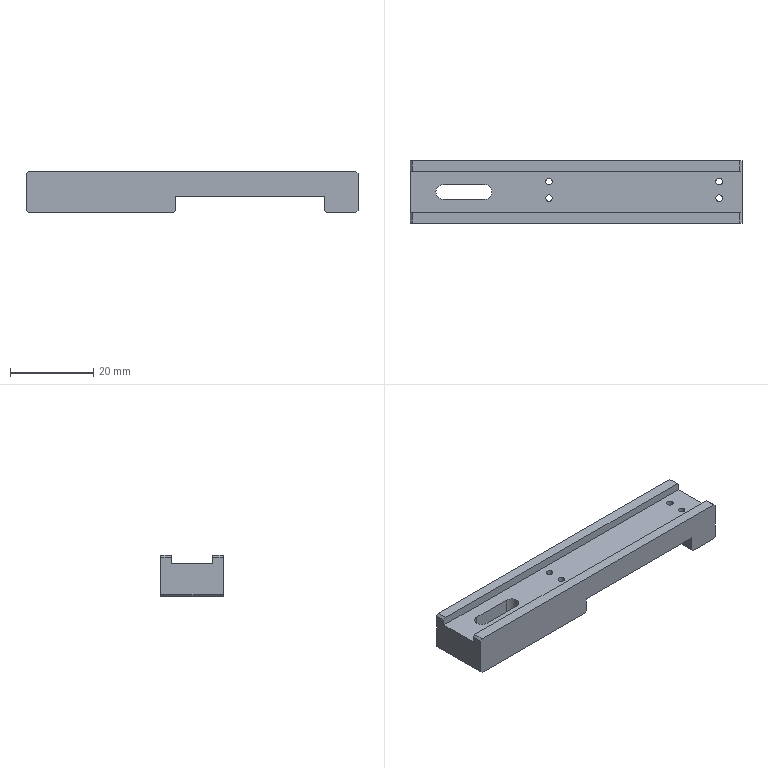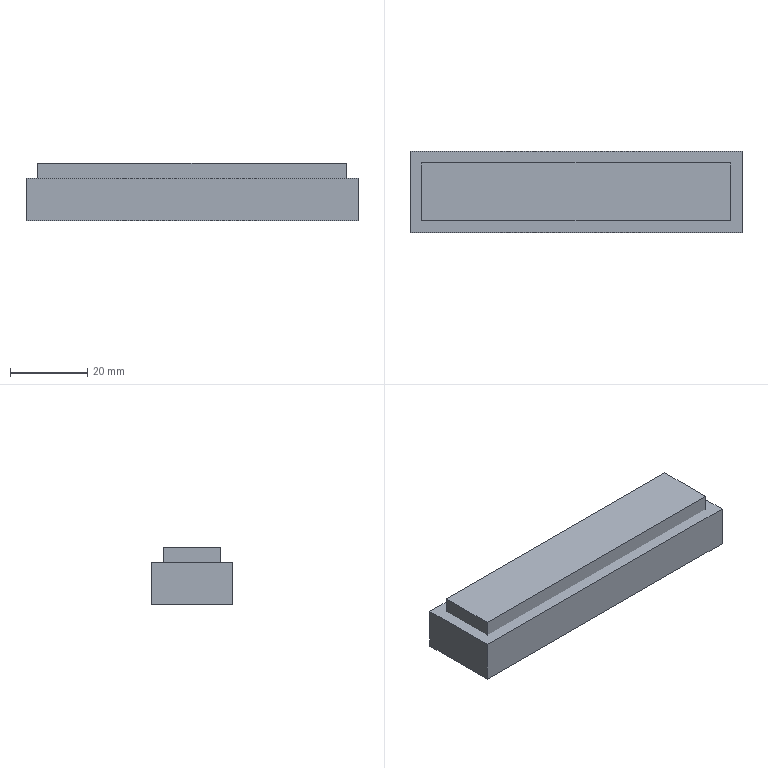CAM job | NX | 3-axis milling, drilling | part box 80 x 15 x 10 mm | stock box 86 x 21 x 15 mm
Tools:
number,name,description,diameter,corner_radius,flute_length,length,flutes
3,D63,Milling Tool-5 Parameters,63.0,0.0,50.0,75.0,2
4,D10,Milling Tool-5 Parameters,10.0,0.0,50.0,75.0,2
14,D10JING,Milling Tool-5 Parameters,10.0,0.0,50.0,75.0,2
1,D6A45,Milling Tool-5 Parameters,6.0,0.0,50.0,75.0,2
24,1.6ZT,Drilling Tool,1.6,0.0,35.0,50.0,2
17,D3,Milling Tool-5 Parameters,3.0,0.0,50.0,75.0,2
16,D6,Milling Tool-5 Parameters,6.0,0.0,50.0,75.0,2
Operations:
program,operation,operation_type,tool,method,geometry_group,spindle_rpm,surface_speed,feed_per_tooth,feed_cut,feed_plunge,cut_length_mm,path_length_mm,cut_time_min,machine_time_min
1,FLOOR_WALL,VolumeBased25DMillingOperation,D63,METHOD,A,6500.0,1286.0,0.1154,1500.0,100.0,161.0,215.0,0.1073,0.1127
1,DRILLING,Operation,D6A45,METHOD,A,5000.0,94.0,0.025,250.0,0.0,16.2,152.51,0.0648,0.0784
1,DRILLING_COPY_1_COPY,Operation,1.6ZT,METHOD,A,2000.0,37.0,0.0375,150.0,0.0,51.923,223.955,0.3462,0.3634
1,ADAPTIVE_MILLING,CavityMilling,D10,METHOD,A,7500.0,235.0,0.2,3000.0,1000.0,2724.517,2881.399,0.9122,0.9279
1,ZLEVEL_PROFILE,ZLevelMilling,D10JING,METHOD,A,7500.0,235.0,0.0667,1000.0,100.0,228.754,306.754,0.2288,0.2366
1,FLOOR_WALL_1_COPY_COPY,VolumeBased25DMillingOperation,D10JING,METHOD,A,7500.0,235.0,0.08,1200.0,1000.0,260.997,473.497,0.2205,0.2417
1,ZLEVEL_PROFILE_1,ZLevelMilling,D3,METHOD,A,7500.0,70.0,0.08,1200.0,1000.0,897.389,963.389,0.7516,0.7582
1,PLANAR_MILL,PlanarMilling,D6A45,METHOD,A,7500.0,141.0,0.0833,1250.0,100.0,201.886,448.765,0.1615,0.1862
1,PLANAR_MILL_COPY,PlanarMilling,D6A45,METHOD,A,7500.0,141.0,0.0833,1250.0,100.0,73.381,225.244,0.0587,0.0739
2,FLOOR_WALL_COPY,VolumeBased25DMillingOperation,D63,METHOD,B,6500.0,1286.0,0.1154,1500.0,100.0,775.0,1621.001,0.5167,0.6013
2,ZLEVEL_PROFILE_1_COPY_COPY,ZLevelMilling,D6,METHOD,B,7500.0,141.0,0.11,1650.0,1000.0,784.303,845.003,0.4767,0.4828
2,PLANAR_MILL_COPY_1,PlanarMilling,D6A45,METHOD,B,7500.0,141.0,0.0833,1250.0,100.0,352.8,486.315,0.2822,0.2956
2,刀补16,ZLevelMilling,D6,METHOD,B,7500.0,141.0,0.0667,1000.0,1000.0,191.79,309.339,0.1918,0.2035